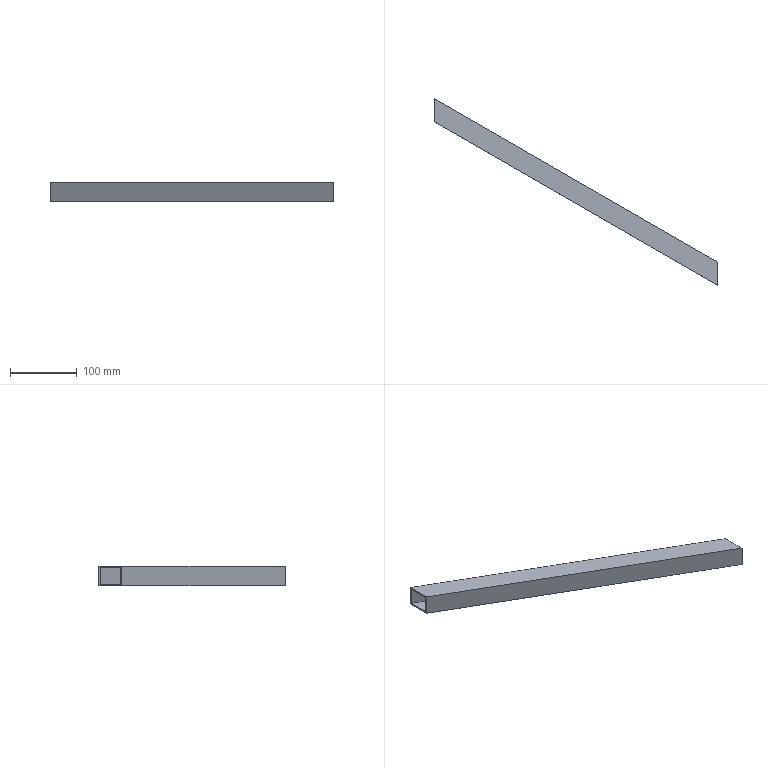Part | NX | features solid 2 | 1 solid | 10 faces | box 425 x 280.015 x 30 mm | volume 109927 mm3 | plane 10
STEP:
#1=CARTESIAN_POINT('',(665.,-264.989,-103.));
#2=VERTEX_POINT('',#1);
#3=CARTESIAN_POINT('',(665.,-264.989,-77.));
#4=VERTEX_POINT('',#3);
#5=CARTESIAN_POINT('',(665.,-264.989,-105.));
#6=DIRECTION('',(0.,0.,-1.));
#7=VECTOR('',#6,1000.);
#8=LINE('',#5,#7);
#9=EDGE_CURVE('',#2,#4,#8,.F.);
#10=ORIENTED_EDGE('',*,*,#9,.T.);
#11=CARTESIAN_POINT('',(240.,-19.615,-77.));
#12=VERTEX_POINT('',#11);
#13=CARTESIAN_POINT('',(475.795,-155.751,-77.));
#14=DIRECTION('',(0.866,-0.5,0.));
#15=VECTOR('',#14,1000.);
#16=LINE('',#13,#15);
#17=EDGE_CURVE('',#12,#4,#16,.T.);
#18=ORIENTED_EDGE('',*,*,#17,.F.);
#19=CARTESIAN_POINT('',(240.,-19.615,-103.));
#20=VERTEX_POINT('',#19);
#21=CARTESIAN_POINT('',(240.,-19.615,-105.));
#22=DIRECTION('',(0.,0.,-1.));
#23=VECTOR('',#22,1000.);
#24=LINE('',#21,#23);
#25=EDGE_CURVE('',#20,#12,#24,.F.);
#26=ORIENTED_EDGE('',*,*,#25,.F.);
#27=CARTESIAN_POINT('',(475.795,-155.751,-103.));
#28=DIRECTION('',(0.866,-0.5,0.));
#29=VECTOR('',#28,1000.);
#30=LINE('',#27,#29);
#31=EDGE_CURVE('',#20,#2,#30,.T.);
#32=ORIENTED_EDGE('',*,*,#31,.T.);
#33=EDGE_LOOP('',(#10,#18,#26,#32));
#34=FACE_BOUND('',#33,.T.);
#35=CARTESIAN_POINT('',(475.795,-155.751,-105.));
#36=DIRECTION('',(0.5,0.866,0.));
#37=DIRECTION('',(0.,0.,-1.));
#38=AXIS2_PLACEMENT_3D('',#35,#36,#37);
#39=PLANE('',#38);
#40=ADVANCED_FACE('',(#34),#39,.F.);
#41=CARTESIAN_POINT('',(665.,-295.011,-77.));
#42=VERTEX_POINT('',#41);
#43=CARTESIAN_POINT('',(665.,-435.477,-77.));
#44=DIRECTION('',(0.,1.,0.));
#45=VECTOR('',#44,1000.);
#46=LINE('',#43,#45);
#47=EDGE_CURVE('',#4,#42,#46,.F.);
#48=ORIENTED_EDGE('',*,*,#47,.T.);
#49=CARTESIAN_POINT('',(240.,-49.637,-77.));
#50=VERTEX_POINT('',#49);
#51=CARTESIAN_POINT('',(462.795,-178.268,-77.));
#52=DIRECTION('',(0.866,-0.5,0.));
#53=VECTOR('',#52,1000.);
#54=LINE('',#51,#53);
#55=EDGE_CURVE('',#50,#42,#54,.T.);
#56=ORIENTED_EDGE('',*,*,#55,.F.);
#57=CARTESIAN_POINT('',(240.,-435.477,-77.));
#58=DIRECTION('',(0.,1.,0.));
#59=VECTOR('',#58,1000.);
#60=LINE('',#57,#59);
#61=EDGE_CURVE('',#12,#50,#60,.F.);
#62=ORIENTED_EDGE('',*,*,#61,.F.);
#63=ORIENTED_EDGE('',*,*,#17,.T.);
#64=EDGE_LOOP('',(#48,#56,#62,#63));
#65=FACE_BOUND('',#64,.T.);
#66=CARTESIAN_POINT('',(314.295,-435.477,-77.));
#67=DIRECTION('',(0.,0.,1.));
#68=DIRECTION('',(0.5,0.866,0.));
#69=AXIS2_PLACEMENT_3D('',#66,#67,#68);
#70=PLANE('',#69);
#71=ADVANCED_FACE('',(#65),#70,.F.);
#72=CARTESIAN_POINT('',(665.,-295.011,-103.));
#73=VERTEX_POINT('',#72);
#74=CARTESIAN_POINT('',(665.,-295.011,-105.));
#75=DIRECTION('',(0.,0.,-1.));
#76=VECTOR('',#75,1000.);
#77=LINE('',#74,#76);
#78=EDGE_CURVE('',#73,#42,#77,.F.);
#79=ORIENTED_EDGE('',*,*,#78,.F.);
#80=CARTESIAN_POINT('',(240.,-49.637,-103.));
#81=VERTEX_POINT('',#80);
#82=CARTESIAN_POINT('',(462.795,-178.268,-103.));
#83=DIRECTION('',(0.866,-0.5,0.));
#84=VECTOR('',#83,1000.);
#85=LINE('',#82,#84);
#86=EDGE_CURVE('',#81,#73,#85,.T.);
#87=ORIENTED_EDGE('',*,*,#86,.F.);
#88=CARTESIAN_POINT('',(240.,-49.637,-105.));
#89=DIRECTION('',(0.,0.,-1.));
#90=VECTOR('',#89,1000.);
#91=LINE('',#88,#90);
#92=EDGE_CURVE('',#81,#50,#91,.F.);
#93=ORIENTED_EDGE('',*,*,#92,.T.);
#94=ORIENTED_EDGE('',*,*,#55,.T.);
#95=EDGE_LOOP('',(#79,#87,#93,#94));
#96=FACE_BOUND('',#95,.T.);
#97=CARTESIAN_POINT('',(462.795,-178.268,-105.));
#98=DIRECTION('',(0.5,0.866,0.));
#99=DIRECTION('',(0.,0.,-1.));
#100=AXIS2_PLACEMENT_3D('',#97,#98,#99);
#101=PLANE('',#100);
#102=ADVANCED_FACE('',(#96),#101,.T.);
#103=CARTESIAN_POINT('',(665.,-262.679,-75.));
#104=VERTEX_POINT('',#103);
#105=CARTESIAN_POINT('',(665.,-297.321,-75.));
#106=VERTEX_POINT('',#105);
#107=CARTESIAN_POINT('',(665.,-435.477,-75.));
#108=DIRECTION('',(0.,1.,0.));
#109=VECTOR('',#108,1000.);
#110=LINE('',#107,#109);
#111=EDGE_CURVE('',#104,#106,#110,.F.);
#112=ORIENTED_EDGE('',*,*,#111,.F.);
#113=CARTESIAN_POINT('',(240.,-17.306,-75.));
#114=VERTEX_POINT('',#113);
#115=CARTESIAN_POINT('',(476.795,-154.019,-75.));
#116=DIRECTION('',(0.866,-0.5,0.));
#117=VECTOR('',#116,1000.);
#118=LINE('',#115,#117);
#119=EDGE_CURVE('',#114,#104,#118,.T.);
#120=ORIENTED_EDGE('',*,*,#119,.F.);
#121=CARTESIAN_POINT('',(240.,-51.947,-75.));
#122=VERTEX_POINT('',#121);
#123=CARTESIAN_POINT('',(240.,-435.477,-75.));
#124=DIRECTION('',(0.,1.,0.));
#125=VECTOR('',#124,1000.);
#126=LINE('',#123,#125);
#127=EDGE_CURVE('',#114,#122,#126,.F.);
#128=ORIENTED_EDGE('',*,*,#127,.T.);
#129=CARTESIAN_POINT('',(461.795,-180.,-75.));
#130=DIRECTION('',(0.866,-0.5,0.));
#131=VECTOR('',#130,1000.);
#132=LINE('',#129,#131);
#133=EDGE_CURVE('',#122,#106,#132,.T.);
#134=ORIENTED_EDGE('',*,*,#133,.T.);
#135=EDGE_LOOP('',(#112,#120,#128,#134));
#136=FACE_BOUND('',#135,.T.);
#137=CARTESIAN_POINT('',(314.295,-435.477,-75.));
#138=DIRECTION('',(0.,0.,1.));
#139=DIRECTION('',(0.5,0.866,0.));
#140=AXIS2_PLACEMENT_3D('',#137,#138,#139);
#141=PLANE('',#140);
#142=ADVANCED_FACE('',(#136),#141,.T.);
#143=CARTESIAN_POINT('',(665.,-262.679,-105.));
#144=VERTEX_POINT('',#143);
#145=CARTESIAN_POINT('',(665.,-262.679,-105.));
#146=DIRECTION('',(0.,0.,-1.));
#147=VECTOR('',#146,1000.);
#148=LINE('',#145,#147);
#149=EDGE_CURVE('',#144,#104,#148,.F.);
#150=ORIENTED_EDGE('',*,*,#149,.F.);
#151=CARTESIAN_POINT('',(240.,-17.306,-105.));
#152=VERTEX_POINT('',#151);
#153=CARTESIAN_POINT('',(476.795,-154.019,-105.));
#154=DIRECTION('',(0.866,-0.5,0.));
#155=VECTOR('',#154,1000.);
#156=LINE('',#153,#155);
#157=EDGE_CURVE('',#152,#144,#156,.T.);
#158=ORIENTED_EDGE('',*,*,#157,.F.);
#159=CARTESIAN_POINT('',(240.,-17.306,-105.));
#160=DIRECTION('',(0.,0.,-1.));
#161=VECTOR('',#160,1000.);
#162=LINE('',#159,#161);
#163=EDGE_CURVE('',#152,#114,#162,.F.);
#164=ORIENTED_EDGE('',*,*,#163,.T.);
#165=ORIENTED_EDGE('',*,*,#119,.T.);
#166=EDGE_LOOP('',(#150,#158,#164,#165));
#167=FACE_BOUND('',#166,.T.);
#168=CARTESIAN_POINT('',(476.795,-154.019,-105.));
#169=DIRECTION('',(0.5,0.866,0.));
#170=DIRECTION('',(0.,0.,-1.));
#171=AXIS2_PLACEMENT_3D('',#168,#169,#170);
#172=PLANE('',#171);
#173=ADVANCED_FACE('',(#167),#172,.T.);
#174=CARTESIAN_POINT('',(665.,-297.321,-105.));
#175=VERTEX_POINT('',#174);
#176=CARTESIAN_POINT('',(665.,-435.477,-105.));
#177=DIRECTION('',(0.,1.,0.));
#178=VECTOR('',#177,1000.);
#179=LINE('',#176,#178);
#180=EDGE_CURVE('',#144,#175,#179,.F.);
#181=ORIENTED_EDGE('',*,*,#180,.T.);
#182=CARTESIAN_POINT('',(240.,-51.947,-105.));
#183=VERTEX_POINT('',#182);
#184=CARTESIAN_POINT('',(461.795,-180.,-105.));
#185=DIRECTION('',(0.866,-0.5,0.));
#186=VECTOR('',#185,1000.);
#187=LINE('',#184,#186);
#188=EDGE_CURVE('',#183,#175,#187,.T.);
#189=ORIENTED_EDGE('',*,*,#188,.F.);
#190=CARTESIAN_POINT('',(240.,-435.477,-105.));
#191=DIRECTION('',(0.,1.,0.));
#192=VECTOR('',#191,1000.);
#193=LINE('',#190,#192);
#194=EDGE_CURVE('',#152,#183,#193,.F.);
#195=ORIENTED_EDGE('',*,*,#194,.F.);
#196=ORIENTED_EDGE('',*,*,#157,.T.);
#197=EDGE_LOOP('',(#181,#189,#195,#196));
#198=FACE_BOUND('',#197,.T.);
#199=CARTESIAN_POINT('',(314.295,-435.477,-105.));
#200=DIRECTION('',(0.,0.,1.));
#201=DIRECTION('',(0.5,0.866,0.));
#202=AXIS2_PLACEMENT_3D('',#199,#200,#201);
#203=PLANE('',#202);
#204=ADVANCED_FACE('',(#198),#203,.F.);
#205=CARTESIAN_POINT('',(665.,-297.321,-105.));
#206=DIRECTION('',(0.,0.,-1.));
#207=VECTOR('',#206,1000.);
#208=LINE('',#205,#207);
#209=EDGE_CURVE('',#175,#106,#208,.F.);
#210=ORIENTED_EDGE('',*,*,#209,.T.);
#211=ORIENTED_EDGE('',*,*,#133,.F.);
#212=CARTESIAN_POINT('',(240.,-51.947,-105.));
#213=DIRECTION('',(0.,0.,-1.));
#214=VECTOR('',#213,1000.);
#215=LINE('',#212,#214);
#216=EDGE_CURVE('',#183,#122,#215,.F.);
#217=ORIENTED_EDGE('',*,*,#216,.F.);
#218=ORIENTED_EDGE('',*,*,#188,.T.);
#219=EDGE_LOOP('',(#210,#211,#217,#218));
#220=FACE_BOUND('',#219,.T.);
#221=CARTESIAN_POINT('',(461.795,-180.,-105.));
#222=DIRECTION('',(0.5,0.866,0.));
#223=DIRECTION('',(0.,0.,-1.));
#224=AXIS2_PLACEMENT_3D('',#221,#222,#223);
#225=PLANE('',#224);
#226=ADVANCED_FACE('',(#220),#225,.F.);
#227=CARTESIAN_POINT('',(665.,-435.477,-103.));
#228=DIRECTION('',(0.,1.,0.));
#229=VECTOR('',#228,1000.);
#230=LINE('',#227,#229);
#231=EDGE_CURVE('',#2,#73,#230,.F.);
#232=ORIENTED_EDGE('',*,*,#231,.F.);
#233=ORIENTED_EDGE('',*,*,#31,.F.);
#234=CARTESIAN_POINT('',(240.,-435.477,-103.));
#235=DIRECTION('',(0.,1.,0.));
#236=VECTOR('',#235,1000.);
#237=LINE('',#234,#236);
#238=EDGE_CURVE('',#20,#81,#237,.F.);
#239=ORIENTED_EDGE('',*,*,#238,.T.);
#240=ORIENTED_EDGE('',*,*,#86,.T.);
#241=EDGE_LOOP('',(#232,#233,#239,#240));
#242=FACE_BOUND('',#241,.T.);
#243=CARTESIAN_POINT('',(314.295,-435.477,-103.));
#244=DIRECTION('',(0.,0.,1.));
#245=DIRECTION('',(0.5,0.866,0.));
#246=AXIS2_PLACEMENT_3D('',#243,#244,#245);
#247=PLANE('',#246);
#248=ADVANCED_FACE('',(#242),#247,.T.);
#249=ORIENTED_EDGE('',*,*,#127,.F.);
#250=ORIENTED_EDGE('',*,*,#163,.F.);
#251=ORIENTED_EDGE('',*,*,#194,.T.);
#252=ORIENTED_EDGE('',*,*,#216,.T.);
#253=EDGE_LOOP('',(#249,#250,#251,#252));
#254=FACE_BOUND('',#253,.T.);
#255=ORIENTED_EDGE('',*,*,#25,.T.);
#256=ORIENTED_EDGE('',*,*,#61,.T.);
#257=ORIENTED_EDGE('',*,*,#92,.F.);
#258=ORIENTED_EDGE('',*,*,#238,.F.);
#259=EDGE_LOOP('',(#255,#256,#257,#258));
#260=FACE_BOUND('',#259,.T.);
#261=CARTESIAN_POINT('',(240.,40.,-75.));
#262=DIRECTION('',(1.,0.,0.));
#263=DIRECTION('',(0.,1.,0.));
#264=AXIS2_PLACEMENT_3D('',#261,#262,#263);
#265=PLANE('',#264);
#266=ADVANCED_FACE('',(#254,#260),#265,.F.);
#267=ORIENTED_EDGE('',*,*,#111,.T.);
#268=ORIENTED_EDGE('',*,*,#209,.F.);
#269=ORIENTED_EDGE('',*,*,#180,.F.);
#270=ORIENTED_EDGE('',*,*,#149,.T.);
#271=EDGE_LOOP('',(#267,#268,#269,#270));
#272=FACE_BOUND('',#271,.T.);
#273=ORIENTED_EDGE('',*,*,#9,.F.);
#274=ORIENTED_EDGE('',*,*,#231,.T.);
#275=ORIENTED_EDGE('',*,*,#78,.T.);
#276=ORIENTED_EDGE('',*,*,#47,.F.);
#277=EDGE_LOOP('',(#273,#274,#275,#276));
#278=FACE_BOUND('',#277,.T.);
#279=CARTESIAN_POINT('',(665.,-588.785,-135.));
#280=DIRECTION('',(1.,0.,0.));
#281=DIRECTION('',(0.,0.,-1.));
#282=AXIS2_PLACEMENT_3D('',#279,#280,#281);
#283=PLANE('',#282);
#284=ADVANCED_FACE('',(#272,#278),#283,.T.);
#285=CLOSED_SHELL('',(#40,#71,#102,#142,#173,#204,#226,#248,#266,#284));
#286=MANIFOLD_SOLID_BREP('',#285);
#287=(LENGTH_UNIT()NAMED_UNIT(*)SI_UNIT(.MILLI.,.METRE.));
#288=UNCERTAINTY_MEASURE_WITH_UNIT(LENGTH_MEASURE(0.00001),#287,'','');
#289=(NAMED_UNIT(*)PLANE_ANGLE_UNIT()SI_UNIT($,.RADIAN.));
#290=(NAMED_UNIT(*)SI_UNIT($,.STERADIAN.)SOLID_ANGLE_UNIT());
#291=(GEOMETRIC_REPRESENTATION_CONTEXT(3)GLOBAL_UNCERTAINTY_ASSIGNED_CONTEXT((#288))GLOBAL_UNIT_ASSIGNED_CONTEXT((#287,#289,#290))REPRESENTATION_CONTEXT('',''));
#292=ADVANCED_BREP_SHAPE_REPRESENTATION('',(#286),#291);